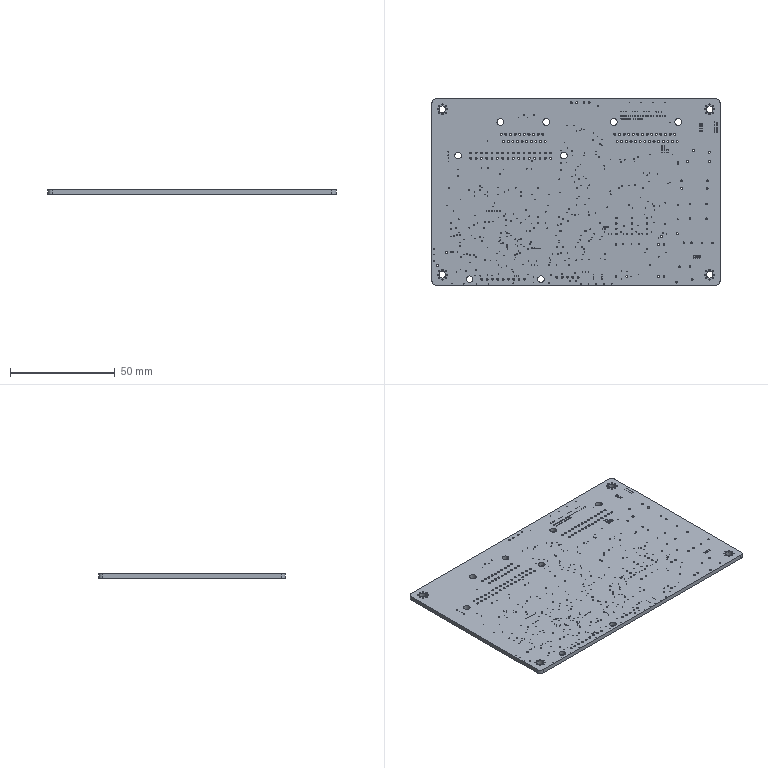Part | SolidWorks | features BaseBody 1 | 1 solid | 1314 faces | box 137.5 x 89 x 2 mm | volume 24002 mm3 | cylinder 1308 | plane 6 | commonest cylinder face diameters 0.305 x890 0.889 x112 1 x100 0.6 x64 0.381 x40 0.8 x28